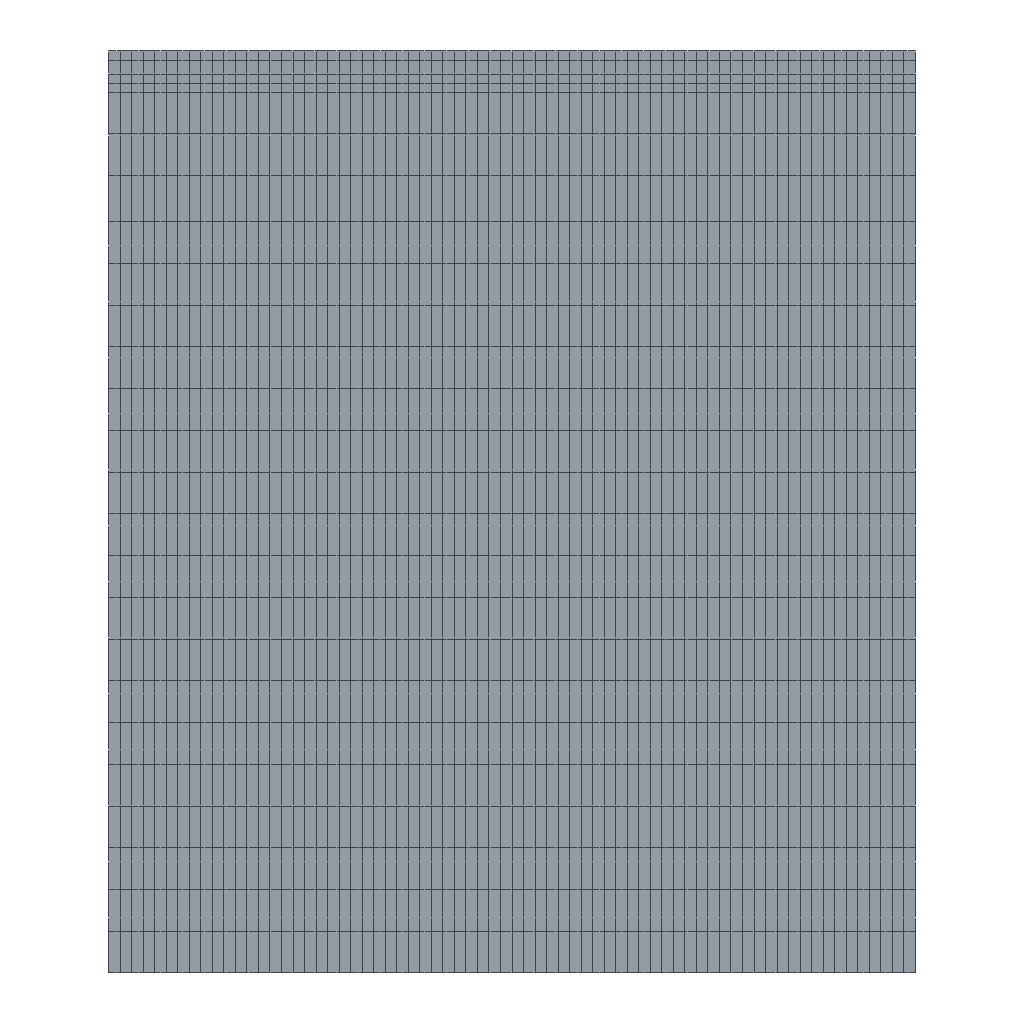Simulation study | abaqus
Set-up summary:
category,name,step,type,value,unit,region
solver,abaqus
solver,version,,,Abaqus/Standard 2020
units,not stated in the deck,,not stated
analysis,deck,,soils,soils
load_step,Step-1,Step-1,soils
load_step,requested,,,1
mesh,nodes,,,1846
mesh,elements,,,1750
element_type,CPE4P,,plane,1750
load,load commands in deck,,count,1
bc,support commands in deck,,count,2
material,LAY1,,in results
material,LAY2,,in results
material,LAY3,,in results
material,LAY4,,in results
material,LAY5,,in results
material,LAY6,,in results
check,setup vs results,,match,"per instance, exact: element labels, types and connectivity; labels of the nodes the elements use; coordinates of those nodes at SINGLE_PRECISION in 1 of 1 instance(s)"
Abaqus input file, long lists of numbers shortened:
*Heading
** Job name: Job-2 Model name: Model-1-Copy
** Generated by: Abaqus/CAE 2020
*Preprint, echo=NO, model=NO, history=NO, contact=NO
**
** PARTS
**
*Part, name=road
*Node
      1,           0., -0.04
      2,          3.5, -0.04
** (1844 more lines like these left out)
*Element, type=CPE4P
 1,   1,  15, 152,   4
 2,  15,  16, 151, 152
** (1748 more lines like these left out)
*Nset, nset=Set-5
   1,   2,   3,   4,  15,  16,  17,  18,  19,  20,  21,  22,  23,  24,  25,  26
  27,  28,  29,  30,  31,  32,  33,  34,  35,  36,  37,  38,  39,  40,  41,  42
** (7 more lines like these left out)
*Elset, elset=Set-5, generate
  1,  70,   1
*Nset, nset=Set-6
   1,   2,   5,   6,  15,  16,  17,  18,  19,  20,  21,  22,  23,  24,  25,  26
  27,  28,  29,  30,  31,  32,  33,  34,  35,  36,  37,  38,  39,  40,  41,  42
** (7 more lines like these left out)
*Elset, elset=Set-6, generate
  71,  140,    1
*Nset, nset=Set-7
    5,    6,   11,   12,  153,  154,  155,  156,  157,  158,  159,  160,  161,  162,  163,  164
  165,  166,  167,  168,  169,  170,  171,  172,  173,  174,  175,  176,  177,  178,  179,  180
** (12 more lines like these left out)
*Elset, elset=Set-7, generate
 1401,  1540,     1
*Nset, nset=Set-8
   11,   12,   13,   14,  395,  396,  397,  398,  399,  400,  401,  402,  403,  404,  405,  406
  407,  408,  409,  410,  411,  412,  413,  414,  415,  416,  417,  418,  419,  420,  421,  422
** (12 more lines like these left out)
*Elset, elset=Set-8, generate
 1611,  1750,     1
*Nset, nset=Set-9
   7,   8,  13,  14, 222, 223, 224, 225, 226, 227, 228, 229, 230, 231, 232, 233
 234, 235, 236, 237, 238, 239, 240, 241, 242, 243, 244, 245, 246, 247, 248, 249
** (7 more lines like these left out)
*Elset, elset=Set-9, generate
 1541,  1610,     1
*Nset, nset=Set-10
    7,    8,    9,   10,  222,  223,  224,  225,  226,  227,  228,  229,  230,  231,  232,  233
  234,  235,  236,  237,  238,  239,  240,  241,  242,  243,  244,  245,  246,  247,  248,  249
** (83 more lines like these left out)
*Elset, elset=Set-10, generate
  141,  1400,     1
** Section: l1
*Solid Section, elset=Set-5, material=lay1
,
** Section: l2
*Solid Section, elset=Set-6, material=lay2
,
** Section: l6
*Solid Section, elset=Set-10, material=lay6
,
** Section: l3
*Solid Section, elset=Set-7, material=lay3
,
** Section: lay5
*Solid Section, elset=Set-9, material=lay5
,
** Section: l4
*Solid Section, elset=Set-8, material=lay4
,
*End Part
**
**
** ASSEMBLY
**
*Assembly, name=Assembly
**
*Instance, name=road-1, part=road
*End Instance
**
*Nset, nset=Set-1, instance=road-1, generate
    1,  1846,     1
*Elset, elset=Set-1, instance=road-1, generate
    1,  1750,     1
*Nset, nset=Set-2, instance=road-1
   9,  10, 308, 309, 310, 311, 312, 313, 314, 315, 316, 317, 318, 319, 320, 321
 322, 323, 324, 325, 326, 327, 328, 329, 330, 331, 332, 333, 334, 335, 336, 337
** (3 more lines like these left out)
*Elset, elset=Set-2, instance=road-1, generate
 1331,  1400,     1
*Nset, nset=Set-3, instance=road-1
   1,   2,   3,   4,   5,   6,   7,   8,   9,  10,  11,  12,  13,  14, 291, 292
 293, 294, 295, 296, 297, 298, 299, 300, 301, 302, 303, 304, 305, 306, 307, 377
** (2 more lines like these left out)
*Elset, elset=Set-3, instance=road-1
    1,   70,   71,  140,  141,  210,  211,  280,  281,  350,  351,  420,  421,  490,  491,  560
  561,  630,  631,  700,  701,  770,  771,  840,  841,  910,  911,  980,  981, 1050, 1051, 1120
** (2 more lines like these left out)
*Nset, nset=Set-4, instance=road-1, generate
    1,  1846,     1
*Elset, elset=Set-4, instance=road-1, generate
    1,  1750,     1
*Nset, nset=Set-5, instance=road-1, generate
    1,  1846,     1
*Elset, elset=Set-5, instance=road-1, generate
    1,  1750,     1
*Nset, nset=Set-6, instance=road-1
   3,   4,  84,  85,  86,  87,  88,  89,  90,  91,  92,  93,  94,  95,  96,  97
  98,  99, 100, 101, 102, 103, 104, 105, 106, 107, 108, 109, 110, 111, 112, 113
** (3 more lines like these left out)
*Elset, elset=Set-6, instance=road-1, generate
  1,  70,   1
*Nset, nset=Set-7, instance=road-1, generate
    1,  1846,     1
*Elset, elset=Set-7, instance=road-1, generate
    1,  1750,     1
*Elset, elset=_Surf-1_S3, internal, instance=road-1, generate
  1,  70,   1
*Surface, type=ELEMENT, name=Surf-1
_Surf-1_S3, S3
*End Assembly
*Amplitude, name=Amp-1
             0.,              0.,            100.,              1.
**
** MATERIALS
**
*Material, name=lay1
*Density
2650.,
*Elastic
 1.4e+09, 0.3
*Gap Flow
 0.001,
*Permeability, specific=9800.
 4.8e-05, 0.2
*Material, name=lay2
*Density
2540.,
*Elastic
 1.2e+09, 0.35
*Gap Flow
 0.001,
*Permeability, specific=9800.
 1.74e-05, 0.2
*Material, name=lay3
*Density
2520.,
*Elastic
 9e+08, 0.35
*Gap Flow
 0.001,
*Permeability, specific=9800.
 1.26e-05, 0.2
*Material, name=lay4
*Density
2190.,
*Elastic
 1.6e+09, 0.2
*Gap Flow
 0.001,
*Permeability, specific=9800.
 1.22e-07, 0.2
*Material, name=lay5
*Density
2190.,
*Elastic
 3.5e+08, 0.3
*Gap Flow
 0.001,
*Permeability, specific=9800.
 0.00027, 0.2
*Material, name=lay6
*Density
1630.,
*Elastic
 4e+07, 0.4
*Gap Flow
 0.001,
*Permeability, specific=9800.
 3.3e-09, 0.2
**
** BOUNDARY CONDITIONS
**
** Name: BC-1 Type: 位移/转角
*Boundary
Set-2, 2, 2
** Name: BC-2 Type: 位移/转角
*Boundary
Set-3, 1, 1
**
** PREDEFINED FIELDS
**
** Name: Predefined Field-2   Type: Pore pressure
*Initial Conditions, TYPE=PORE PRESSURE
Set-4, -3e+06
** Name: Predefined Field-3   Type: Void ratio
*Initial Conditions, TYPE=RATIO
Set-5, 0.2
** ----------------------------------------------------------------
**
** STEP: Step-1
**
*Step, name=Step-1, nlgeom=YES, inc=10000, unsymm=YES
*Soils, consolidation, end=PERIOD, stabilize=0.0002, allsdtol=0.05, continue=NO
300., 14400., , ,
**
** LOADS
**
** Name: Load-1   Type: Surface pore fluid
*Dsflow, amplitude=Amp-1
Surf-1, S, 1e-06
**
** OUTPUT REQUESTS
**
*Restart, write, frequency=0
**
** FIELD OUTPUT: F-Output-1
**
*Output, field
*Node Output
CF, POR, RF, U, V
*Element Output, directions=YES
E, FLUVR, LE, MISES, MISESONLY, S, SAT, SSAVG, VOIDR
*Contact Output
PFL, PFLA, PTL, PTLA
**
** HISTORY OUTPUT: H-Output-1
**
*Output, history, variable=PRESELECT
*End Step
Results summary:
result,step,,completed,increments=48 time=14400.0/14400.0
result,analysis,,,"soils, consolidation"
result,last_loadstep,,,1
result,primary field,,,"U, POR"
result,reaction total,,FX,0.0,model units
result,reaction total,,FY,-6061.2,model units
result,reaction total,,FZ,0.0,model units